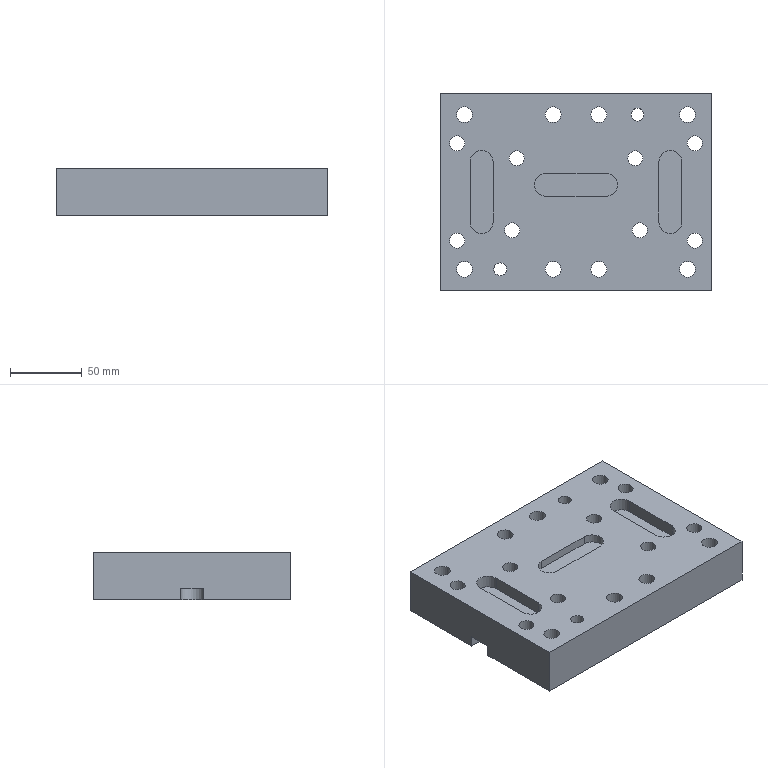Part | STEP file | gslz 2016.10.28-6_id322_x_t | 1 solid | 81 faces | box 190 x 138 x 33 mm | volume 763181 mm3 | cylinder 38 | plane 31 | cone 12 | commonest cylinder face diameters 16 x12 10.5 x8 11 x8 5 x4 6.8 x2 9 x2